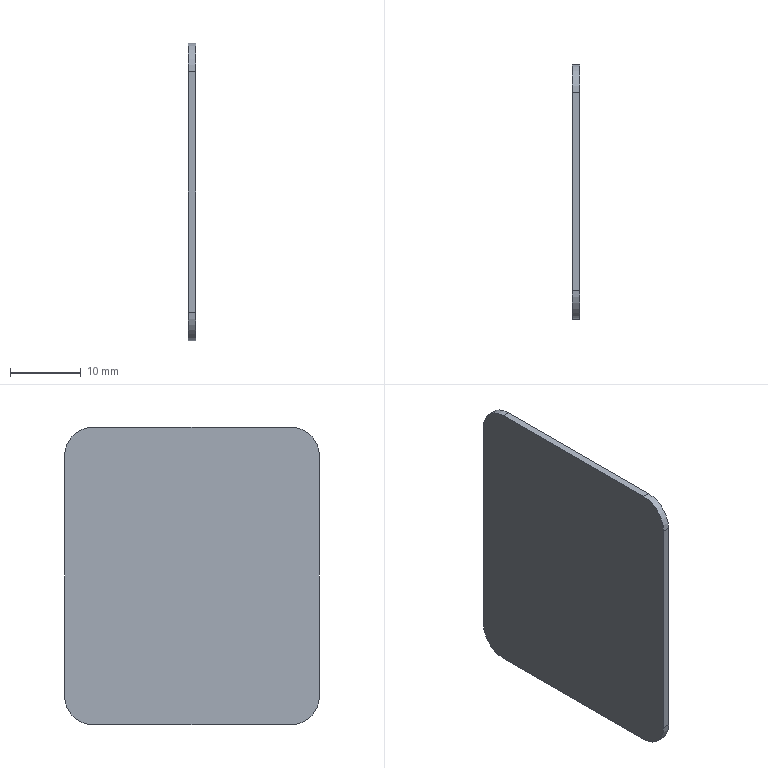Part | STEP file | 1-31.6 | 1 solid | 10 faces | box 1 x 36 x 42 mm | volume 1498 mm3 | plane 6 | cylinder 4 | commonest cylinder face diameters 8 x4
STEP:
#1=CARTESIAN_POINT('',(0.,0.,0.));
#2=DIRECTION('',(0.,0.,1.));
#3=DIRECTION('',(1.,0.,0.));
#4=AXIS2_PLACEMENT_3D('',#1,#2,#3);
#5=CARTESIAN_POINT('',(0.,18.,-17.));
#6=VERTEX_POINT('',#5);
#7=CARTESIAN_POINT('',(0.,18.,17.));
#8=VERTEX_POINT('',#7);
#9=CARTESIAN_POINT('',(0.,18.,-17.));
#10=DIRECTION('',(0.,0.,1.));
#11=VECTOR('',#10,1.);
#12=LINE('',#9,#11);
#13=CARTESIAN_POINT('',(0.,3.,0.));
#14=DIRECTION('',(1.,0.,0.));
#15=DIRECTION('',(0.,1.,0.));
#16=AXIS2_PLACEMENT_3D('',#13,#14,#15);
#17=PLANE('',#16);
#18=CARTESIAN_POINT('',(15.,-17.));
#19=DIRECTION('',(0.,1.));
#20=VECTOR('',#19,1.);
#21=LINE('',#18,#20);
#22=(GEOMETRIC_REPRESENTATION_CONTEXT(2)PARAMETRIC_REPRESENTATION_CONTEXT()REPRESENTATION_CONTEXT('',''));
#23=DEFINITIONAL_REPRESENTATION('',(#21),#22);
#24=PCURVE('',#17,#23);
#25=CARTESIAN_POINT('',(-0.5,18.,0.));
#26=DIRECTION('',(0.,-1.,0.));
#27=DIRECTION('',(0.,0.,1.));
#28=AXIS2_PLACEMENT_3D('',#25,#26,#27);
#29=PLANE('',#28);
#30=CARTESIAN_POINT('',(-17.,-0.5));
#31=DIRECTION('',(1.,0.));
#32=VECTOR('',#31,1.);
#33=LINE('',#30,#32);
#34=(GEOMETRIC_REPRESENTATION_CONTEXT(2)PARAMETRIC_REPRESENTATION_CONTEXT()REPRESENTATION_CONTEXT('',''));
#35=DEFINITIONAL_REPRESENTATION('',(#33),#34);
#36=PCURVE('',#29,#35);
#37=SURFACE_CURVE('',#12,(#24,#36),.PCURVE_S1.);
#38=EDGE_CURVE('',#6,#8,#37,.T.);
#39=ORIENTED_EDGE('',*,*,#38,.T.);
#40=CARTESIAN_POINT('',(0.,14.,21.));
#41=VERTEX_POINT('',#40);
#42=CARTESIAN_POINT('',(0.,14.,17.));
#43=DIRECTION('',(1.,0.,0.));
#44=DIRECTION('',(0.,1.,0.));
#45=AXIS2_PLACEMENT_3D('',#42,#43,#44);
#46=CIRCLE('',#45,4.);
#47=CARTESIAN_POINT('',(11.,17.));
#48=DIRECTION('',(1.,0.));
#49=AXIS2_PLACEMENT_2D('',#47,#48);
#50=CIRCLE('',#49,4.);
#51=(GEOMETRIC_REPRESENTATION_CONTEXT(2)PARAMETRIC_REPRESENTATION_CONTEXT()REPRESENTATION_CONTEXT('',''));
#52=DEFINITIONAL_REPRESENTATION('',(#50),#51);
#53=PCURVE('',#17,#52);
#54=CARTESIAN_POINT('',(0.,14.,17.));
#55=DIRECTION('',(-1.,0.,0.));
#56=DIRECTION('',(0.,1.,0.));
#57=AXIS2_PLACEMENT_3D('',#54,#55,#56);
#58=CYLINDRICAL_SURFACE('',#57,4.);
#59=CARTESIAN_POINT('',(6.283,0.));
#60=DIRECTION('',(-1.,0.));
#61=VECTOR('',#60,1.);
#62=LINE('',#59,#61);
#63=(GEOMETRIC_REPRESENTATION_CONTEXT(2)PARAMETRIC_REPRESENTATION_CONTEXT()REPRESENTATION_CONTEXT('',''));
#64=DEFINITIONAL_REPRESENTATION('',(#62),#63);
#65=PCURVE('',#58,#64);
#66=SURFACE_CURVE('',#46,(#53,#65),.PCURVE_S1.);
#67=EDGE_CURVE('',#8,#41,#66,.T.);
#68=ORIENTED_EDGE('',*,*,#67,.T.);
#69=CARTESIAN_POINT('',(0.,-14.,21.));
#70=VERTEX_POINT('',#69);
#71=CARTESIAN_POINT('',(0.,14.,21.));
#72=DIRECTION('',(0.,-1.,0.));
#73=VECTOR('',#72,1.);
#74=LINE('',#71,#73);
#75=CARTESIAN_POINT('',(11.,21.));
#76=DIRECTION('',(-1.,0.));
#77=VECTOR('',#76,1.);
#78=LINE('',#75,#77);
#79=(GEOMETRIC_REPRESENTATION_CONTEXT(2)PARAMETRIC_REPRESENTATION_CONTEXT()REPRESENTATION_CONTEXT('',''));
#80=DEFINITIONAL_REPRESENTATION('',(#78),#79);
#81=PCURVE('',#17,#80);
#82=CARTESIAN_POINT('',(-0.5,0.,21.));
#83=DIRECTION('',(0.,0.,-1.));
#84=DIRECTION('',(0.,-1.,0.));
#85=AXIS2_PLACEMENT_3D('',#82,#83,#84);
#86=PLANE('',#85);
#87=CARTESIAN_POINT('',(-14.,-0.5));
#88=DIRECTION('',(1.,0.));
#89=VECTOR('',#88,1.);
#90=LINE('',#87,#89);
#91=(GEOMETRIC_REPRESENTATION_CONTEXT(2)PARAMETRIC_REPRESENTATION_CONTEXT()REPRESENTATION_CONTEXT('',''));
#92=DEFINITIONAL_REPRESENTATION('',(#90),#91);
#93=PCURVE('',#86,#92);
#94=SURFACE_CURVE('',#74,(#81,#93),.PCURVE_S1.);
#95=EDGE_CURVE('',#41,#70,#94,.T.);
#96=ORIENTED_EDGE('',*,*,#95,.T.);
#97=CARTESIAN_POINT('',(0.,-18.,17.));
#98=VERTEX_POINT('',#97);
#99=CARTESIAN_POINT('',(0.,-14.,17.));
#100=DIRECTION('',(1.,0.,0.));
#101=DIRECTION('',(0.,0.,1.));
#102=AXIS2_PLACEMENT_3D('',#99,#100,#101);
#103=CIRCLE('',#102,4.);
#104=CARTESIAN_POINT('',(-17.,17.));
#105=DIRECTION('',(0.,1.));
#106=AXIS2_PLACEMENT_2D('',#104,#105);
#107=CIRCLE('',#106,4.);
#108=(GEOMETRIC_REPRESENTATION_CONTEXT(2)PARAMETRIC_REPRESENTATION_CONTEXT()REPRESENTATION_CONTEXT('',''));
#109=DEFINITIONAL_REPRESENTATION('',(#107),#108);
#110=PCURVE('',#17,#109);
#111=CARTESIAN_POINT('',(0.,-14.,17.));
#112=DIRECTION('',(-1.,0.,0.));
#113=DIRECTION('',(0.,0.,1.));
#114=AXIS2_PLACEMENT_3D('',#111,#112,#113);
#115=CYLINDRICAL_SURFACE('',#114,4.);
#116=CARTESIAN_POINT('',(6.283,0.));
#117=DIRECTION('',(-1.,0.));
#118=VECTOR('',#117,1.);
#119=LINE('',#116,#118);
#120=(GEOMETRIC_REPRESENTATION_CONTEXT(2)PARAMETRIC_REPRESENTATION_CONTEXT()REPRESENTATION_CONTEXT('',''));
#121=DEFINITIONAL_REPRESENTATION('',(#119),#120);
#122=PCURVE('',#115,#121);
#123=SURFACE_CURVE('',#103,(#110,#122),.PCURVE_S1.);
#124=EDGE_CURVE('',#70,#98,#123,.T.);
#125=ORIENTED_EDGE('',*,*,#124,.T.);
#126=CARTESIAN_POINT('',(0.,-18.,-17.));
#127=VERTEX_POINT('',#126);
#128=CARTESIAN_POINT('',(0.,-18.,17.));
#129=DIRECTION('',(0.,0.,-1.));
#130=VECTOR('',#129,1.);
#131=LINE('',#128,#130);
#132=CARTESIAN_POINT('',(-21.,17.));
#133=DIRECTION('',(0.,-1.));
#134=VECTOR('',#133,1.);
#135=LINE('',#132,#134);
#136=(GEOMETRIC_REPRESENTATION_CONTEXT(2)PARAMETRIC_REPRESENTATION_CONTEXT()REPRESENTATION_CONTEXT('',''));
#137=DEFINITIONAL_REPRESENTATION('',(#135),#136);
#138=PCURVE('',#17,#137);
#139=CARTESIAN_POINT('',(-0.5,-18.,0.));
#140=DIRECTION('',(0.,1.,0.));
#141=DIRECTION('',(0.,0.,-1.));
#142=AXIS2_PLACEMENT_3D('',#139,#140,#141);
#143=PLANE('',#142);
#144=CARTESIAN_POINT('',(-17.,-0.5));
#145=DIRECTION('',(1.,0.));
#146=VECTOR('',#145,1.);
#147=LINE('',#144,#146);
#148=(GEOMETRIC_REPRESENTATION_CONTEXT(2)PARAMETRIC_REPRESENTATION_CONTEXT()REPRESENTATION_CONTEXT('',''));
#149=DEFINITIONAL_REPRESENTATION('',(#147),#148);
#150=PCURVE('',#143,#149);
#151=SURFACE_CURVE('',#131,(#138,#150),.PCURVE_S1.);
#152=EDGE_CURVE('',#98,#127,#151,.T.);
#153=ORIENTED_EDGE('',*,*,#152,.T.);
#154=CARTESIAN_POINT('',(0.,-14.,-21.));
#155=VERTEX_POINT('',#154);
#156=CARTESIAN_POINT('',(0.,-14.,-17.));
#157=DIRECTION('',(1.,0.,0.));
#158=DIRECTION('',(0.,-1.,0.));
#159=AXIS2_PLACEMENT_3D('',#156,#157,#158);
#160=CIRCLE('',#159,4.);
#161=CARTESIAN_POINT('',(-17.,-17.));
#162=DIRECTION('',(-1.,0.));
#163=AXIS2_PLACEMENT_2D('',#161,#162);
#164=CIRCLE('',#163,4.);
#165=(GEOMETRIC_REPRESENTATION_CONTEXT(2)PARAMETRIC_REPRESENTATION_CONTEXT()REPRESENTATION_CONTEXT('',''));
#166=DEFINITIONAL_REPRESENTATION('',(#164),#165);
#167=PCURVE('',#17,#166);
#168=CARTESIAN_POINT('',(0.,-14.,-17.));
#169=DIRECTION('',(-1.,0.,0.));
#170=DIRECTION('',(0.,-1.,0.));
#171=AXIS2_PLACEMENT_3D('',#168,#169,#170);
#172=CYLINDRICAL_SURFACE('',#171,4.);
#173=CARTESIAN_POINT('',(6.283,0.));
#174=DIRECTION('',(-1.,0.));
#175=VECTOR('',#174,1.);
#176=LINE('',#173,#175);
#177=(GEOMETRIC_REPRESENTATION_CONTEXT(2)PARAMETRIC_REPRESENTATION_CONTEXT()REPRESENTATION_CONTEXT('',''));
#178=DEFINITIONAL_REPRESENTATION('',(#176),#177);
#179=PCURVE('',#172,#178);
#180=SURFACE_CURVE('',#160,(#167,#179),.PCURVE_S1.);
#181=EDGE_CURVE('',#127,#155,#180,.T.);
#182=ORIENTED_EDGE('',*,*,#181,.T.);
#183=CARTESIAN_POINT('',(0.,14.,-21.));
#184=VERTEX_POINT('',#183);
#185=CARTESIAN_POINT('',(0.,-14.,-21.));
#186=DIRECTION('',(0.,1.,0.));
#187=VECTOR('',#186,1.);
#188=LINE('',#185,#187);
#189=CARTESIAN_POINT('',(-17.,-21.));
#190=DIRECTION('',(1.,0.));
#191=VECTOR('',#190,1.);
#192=LINE('',#189,#191);
#193=(GEOMETRIC_REPRESENTATION_CONTEXT(2)PARAMETRIC_REPRESENTATION_CONTEXT()REPRESENTATION_CONTEXT('',''));
#194=DEFINITIONAL_REPRESENTATION('',(#192),#193);
#195=PCURVE('',#17,#194);
#196=CARTESIAN_POINT('',(-0.5,0.,-21.));
#197=DIRECTION('',(0.,0.,1.));
#198=DIRECTION('',(0.,1.,0.));
#199=AXIS2_PLACEMENT_3D('',#196,#197,#198);
#200=PLANE('',#199);
#201=CARTESIAN_POINT('',(-14.,-0.5));
#202=DIRECTION('',(1.,0.));
#203=VECTOR('',#202,1.);
#204=LINE('',#201,#203);
#205=(GEOMETRIC_REPRESENTATION_CONTEXT(2)PARAMETRIC_REPRESENTATION_CONTEXT()REPRESENTATION_CONTEXT('',''));
#206=DEFINITIONAL_REPRESENTATION('',(#204),#205);
#207=PCURVE('',#200,#206);
#208=SURFACE_CURVE('',#188,(#195,#207),.PCURVE_S1.);
#209=EDGE_CURVE('',#155,#184,#208,.T.);
#210=ORIENTED_EDGE('',*,*,#209,.T.);
#211=CARTESIAN_POINT('',(0.,14.,-17.));
#212=DIRECTION('',(1.,0.,0.));
#213=DIRECTION('',(0.,0.,-1.));
#214=AXIS2_PLACEMENT_3D('',#211,#212,#213);
#215=CIRCLE('',#214,4.);
#216=CARTESIAN_POINT('',(11.,-17.));
#217=DIRECTION('',(0.,-1.));
#218=AXIS2_PLACEMENT_2D('',#216,#217);
#219=CIRCLE('',#218,4.);
#220=(GEOMETRIC_REPRESENTATION_CONTEXT(2)PARAMETRIC_REPRESENTATION_CONTEXT()REPRESENTATION_CONTEXT('',''));
#221=DEFINITIONAL_REPRESENTATION('',(#219),#220);
#222=PCURVE('',#17,#221);
#223=CARTESIAN_POINT('',(0.,14.,-17.));
#224=DIRECTION('',(-1.,0.,0.));
#225=DIRECTION('',(0.,0.,-1.));
#226=AXIS2_PLACEMENT_3D('',#223,#224,#225);
#227=CYLINDRICAL_SURFACE('',#226,4.);
#228=CARTESIAN_POINT('',(6.283,0.));
#229=DIRECTION('',(-1.,0.));
#230=VECTOR('',#229,1.);
#231=LINE('',#228,#230);
#232=(GEOMETRIC_REPRESENTATION_CONTEXT(2)PARAMETRIC_REPRESENTATION_CONTEXT()REPRESENTATION_CONTEXT('',''));
#233=DEFINITIONAL_REPRESENTATION('',(#231),#232);
#234=PCURVE('',#227,#233);
#235=SURFACE_CURVE('',#215,(#222,#234),.PCURVE_S1.);
#236=EDGE_CURVE('',#184,#6,#235,.T.);
#237=ORIENTED_EDGE('',*,*,#236,.T.);
#238=EDGE_LOOP('',(#39,#68,#96,#125,#153,#182,#210,#237));
#239=FACE_BOUND('',#238,.T.);
#240=ADVANCED_FACE('',(#239),#17,.T.);
#241=CARTESIAN_POINT('',(-1.,18.,-17.));
#242=VERTEX_POINT('',#241);
#243=CARTESIAN_POINT('',(-1.,18.,17.));
#244=VERTEX_POINT('',#243);
#245=CARTESIAN_POINT('',(-1.,18.,-17.));
#246=DIRECTION('',(0.,0.,1.));
#247=VECTOR('',#246,1.);
#248=LINE('',#245,#247);
#249=CARTESIAN_POINT('',(-1.,3.,0.));
#250=DIRECTION('',(1.,0.,0.));
#251=DIRECTION('',(0.,1.,0.));
#252=AXIS2_PLACEMENT_3D('',#249,#250,#251);
#253=PLANE('',#252);
#254=CARTESIAN_POINT('',(15.,-17.));
#255=DIRECTION('',(0.,1.));
#256=VECTOR('',#255,1.);
#257=LINE('',#254,#256);
#258=(GEOMETRIC_REPRESENTATION_CONTEXT(2)PARAMETRIC_REPRESENTATION_CONTEXT()REPRESENTATION_CONTEXT('',''));
#259=DEFINITIONAL_REPRESENTATION('',(#257),#258);
#260=PCURVE('',#253,#259);
#261=CARTESIAN_POINT('',(-17.,0.5));
#262=DIRECTION('',(1.,0.));
#263=VECTOR('',#262,1.);
#264=LINE('',#261,#263);
#265=(GEOMETRIC_REPRESENTATION_CONTEXT(2)PARAMETRIC_REPRESENTATION_CONTEXT()REPRESENTATION_CONTEXT('',''));
#266=DEFINITIONAL_REPRESENTATION('',(#264),#265);
#267=PCURVE('',#29,#266);
#268=SURFACE_CURVE('',#248,(#260,#267),.PCURVE_S1.);
#269=EDGE_CURVE('',#242,#244,#268,.T.);
#270=ORIENTED_EDGE('',*,*,#269,.T.);
#271=CARTESIAN_POINT('',(-1.,14.,21.));
#272=VERTEX_POINT('',#271);
#273=CARTESIAN_POINT('',(-1.,14.,17.));
#274=DIRECTION('',(1.,0.,0.));
#275=DIRECTION('',(0.,1.,0.));
#276=AXIS2_PLACEMENT_3D('',#273,#274,#275);
#277=CIRCLE('',#276,4.);
#278=CARTESIAN_POINT('',(11.,17.));
#279=DIRECTION('',(1.,0.));
#280=AXIS2_PLACEMENT_2D('',#278,#279);
#281=CIRCLE('',#280,4.);
#282=(GEOMETRIC_REPRESENTATION_CONTEXT(2)PARAMETRIC_REPRESENTATION_CONTEXT()REPRESENTATION_CONTEXT('',''));
#283=DEFINITIONAL_REPRESENTATION('',(#281),#282);
#284=PCURVE('',#253,#283);
#285=CARTESIAN_POINT('',(6.283,1.));
#286=DIRECTION('',(-1.,0.));
#287=VECTOR('',#286,1.);
#288=LINE('',#285,#287);
#289=(GEOMETRIC_REPRESENTATION_CONTEXT(2)PARAMETRIC_REPRESENTATION_CONTEXT()REPRESENTATION_CONTEXT('',''));
#290=DEFINITIONAL_REPRESENTATION('',(#288),#289);
#291=PCURVE('',#58,#290);
#292=SURFACE_CURVE('',#277,(#284,#291),.PCURVE_S1.);
#293=EDGE_CURVE('',#244,#272,#292,.T.);
#294=ORIENTED_EDGE('',*,*,#293,.T.);
#295=CARTESIAN_POINT('',(-1.,-14.,21.));
#296=VERTEX_POINT('',#295);
#297=CARTESIAN_POINT('',(-1.,14.,21.));
#298=DIRECTION('',(0.,-1.,0.));
#299=VECTOR('',#298,1.);
#300=LINE('',#297,#299);
#301=CARTESIAN_POINT('',(11.,21.));
#302=DIRECTION('',(-1.,0.));
#303=VECTOR('',#302,1.);
#304=LINE('',#301,#303);
#305=(GEOMETRIC_REPRESENTATION_CONTEXT(2)PARAMETRIC_REPRESENTATION_CONTEXT()REPRESENTATION_CONTEXT('',''));
#306=DEFINITIONAL_REPRESENTATION('',(#304),#305);
#307=PCURVE('',#253,#306);
#308=CARTESIAN_POINT('',(-14.,0.5));
#309=DIRECTION('',(1.,0.));
#310=VECTOR('',#309,1.);
#311=LINE('',#308,#310);
#312=(GEOMETRIC_REPRESENTATION_CONTEXT(2)PARAMETRIC_REPRESENTATION_CONTEXT()REPRESENTATION_CONTEXT('',''));
#313=DEFINITIONAL_REPRESENTATION('',(#311),#312);
#314=PCURVE('',#86,#313);
#315=SURFACE_CURVE('',#300,(#307,#314),.PCURVE_S1.);
#316=EDGE_CURVE('',#272,#296,#315,.T.);
#317=ORIENTED_EDGE('',*,*,#316,.T.);
#318=CARTESIAN_POINT('',(-1.,-18.,17.));
#319=VERTEX_POINT('',#318);
#320=CARTESIAN_POINT('',(-1.,-14.,17.));
#321=DIRECTION('',(1.,0.,0.));
#322=DIRECTION('',(0.,0.,1.));
#323=AXIS2_PLACEMENT_3D('',#320,#321,#322);
#324=CIRCLE('',#323,4.);
#325=CARTESIAN_POINT('',(-17.,17.));
#326=DIRECTION('',(0.,1.));
#327=AXIS2_PLACEMENT_2D('',#325,#326);
#328=CIRCLE('',#327,4.);
#329=(GEOMETRIC_REPRESENTATION_CONTEXT(2)PARAMETRIC_REPRESENTATION_CONTEXT()REPRESENTATION_CONTEXT('',''));
#330=DEFINITIONAL_REPRESENTATION('',(#328),#329);
#331=PCURVE('',#253,#330);
#332=CARTESIAN_POINT('',(6.283,1.));
#333=DIRECTION('',(-1.,0.));
#334=VECTOR('',#333,1.);
#335=LINE('',#332,#334);
#336=(GEOMETRIC_REPRESENTATION_CONTEXT(2)PARAMETRIC_REPRESENTATION_CONTEXT()REPRESENTATION_CONTEXT('',''));
#337=DEFINITIONAL_REPRESENTATION('',(#335),#336);
#338=PCURVE('',#115,#337);
#339=SURFACE_CURVE('',#324,(#331,#338),.PCURVE_S1.);
#340=EDGE_CURVE('',#296,#319,#339,.T.);
#341=ORIENTED_EDGE('',*,*,#340,.T.);
#342=CARTESIAN_POINT('',(-1.,-18.,-17.));
#343=VERTEX_POINT('',#342);
#344=CARTESIAN_POINT('',(-1.,-18.,17.));
#345=DIRECTION('',(0.,0.,-1.));
#346=VECTOR('',#345,1.);
#347=LINE('',#344,#346);
#348=CARTESIAN_POINT('',(-21.,17.));
#349=DIRECTION('',(0.,-1.));
#350=VECTOR('',#349,1.);
#351=LINE('',#348,#350);
#352=(GEOMETRIC_REPRESENTATION_CONTEXT(2)PARAMETRIC_REPRESENTATION_CONTEXT()REPRESENTATION_CONTEXT('',''));
#353=DEFINITIONAL_REPRESENTATION('',(#351),#352);
#354=PCURVE('',#253,#353);
#355=CARTESIAN_POINT('',(-17.,0.5));
#356=DIRECTION('',(1.,0.));
#357=VECTOR('',#356,1.);
#358=LINE('',#355,#357);
#359=(GEOMETRIC_REPRESENTATION_CONTEXT(2)PARAMETRIC_REPRESENTATION_CONTEXT()REPRESENTATION_CONTEXT('',''));
#360=DEFINITIONAL_REPRESENTATION('',(#358),#359);
#361=PCURVE('',#143,#360);
#362=SURFACE_CURVE('',#347,(#354,#361),.PCURVE_S1.);
#363=EDGE_CURVE('',#319,#343,#362,.T.);
#364=ORIENTED_EDGE('',*,*,#363,.T.);
#365=CARTESIAN_POINT('',(-1.,-14.,-21.));
#366=VERTEX_POINT('',#365);
#367=CARTESIAN_POINT('',(-1.,-14.,-17.));
#368=DIRECTION('',(1.,0.,0.));
#369=DIRECTION('',(0.,-1.,0.));
#370=AXIS2_PLACEMENT_3D('',#367,#368,#369);
#371=CIRCLE('',#370,4.);
#372=CARTESIAN_POINT('',(-17.,-17.));
#373=DIRECTION('',(-1.,0.));
#374=AXIS2_PLACEMENT_2D('',#372,#373);
#375=CIRCLE('',#374,4.);
#376=(GEOMETRIC_REPRESENTATION_CONTEXT(2)PARAMETRIC_REPRESENTATION_CONTEXT()REPRESENTATION_CONTEXT('',''));
#377=DEFINITIONAL_REPRESENTATION('',(#375),#376);
#378=PCURVE('',#253,#377);
#379=CARTESIAN_POINT('',(6.283,1.));
#380=DIRECTION('',(-1.,0.));
#381=VECTOR('',#380,1.);
#382=LINE('',#379,#381);
#383=(GEOMETRIC_REPRESENTATION_CONTEXT(2)PARAMETRIC_REPRESENTATION_CONTEXT()REPRESENTATION_CONTEXT('',''));
#384=DEFINITIONAL_REPRESENTATION('',(#382),#383);
#385=PCURVE('',#172,#384);
#386=SURFACE_CURVE('',#371,(#378,#385),.PCURVE_S1.);
#387=EDGE_CURVE('',#343,#366,#386,.T.);
#388=ORIENTED_EDGE('',*,*,#387,.T.);
#389=CARTESIAN_POINT('',(-1.,14.,-21.));
#390=VERTEX_POINT('',#389);
#391=CARTESIAN_POINT('',(-1.,-14.,-21.));
#392=DIRECTION('',(0.,1.,0.));
#393=VECTOR('',#392,1.);
#394=LINE('',#391,#393);
#395=CARTESIAN_POINT('',(-17.,-21.));
#396=DIRECTION('',(1.,0.));
#397=VECTOR('',#396,1.);
#398=LINE('',#395,#397);
#399=(GEOMETRIC_REPRESENTATION_CONTEXT(2)PARAMETRIC_REPRESENTATION_CONTEXT()REPRESENTATION_CONTEXT('',''));
#400=DEFINITIONAL_REPRESENTATION('',(#398),#399);
#401=PCURVE('',#253,#400);
#402=CARTESIAN_POINT('',(-14.,0.5));
#403=DIRECTION('',(1.,0.));
#404=VECTOR('',#403,1.);
#405=LINE('',#402,#404);
#406=(GEOMETRIC_REPRESENTATION_CONTEXT(2)PARAMETRIC_REPRESENTATION_CONTEXT()REPRESENTATION_CONTEXT('',''));
#407=DEFINITIONAL_REPRESENTATION('',(#405),#406);
#408=PCURVE('',#200,#407);
#409=SURFACE_CURVE('',#394,(#401,#408),.PCURVE_S1.);
#410=EDGE_CURVE('',#366,#390,#409,.T.);
#411=ORIENTED_EDGE('',*,*,#410,.T.);
#412=CARTESIAN_POINT('',(-1.,14.,-17.));
#413=DIRECTION('',(1.,0.,0.));
#414=DIRECTION('',(0.,0.,-1.));
#415=AXIS2_PLACEMENT_3D('',#412,#413,#414);
#416=CIRCLE('',#415,4.);
#417=CARTESIAN_POINT('',(11.,-17.));
#418=DIRECTION('',(0.,-1.));
#419=AXIS2_PLACEMENT_2D('',#417,#418);
#420=CIRCLE('',#419,4.);
#421=(GEOMETRIC_REPRESENTATION_CONTEXT(2)PARAMETRIC_REPRESENTATION_CONTEXT()REPRESENTATION_CONTEXT('',''));
#422=DEFINITIONAL_REPRESENTATION('',(#420),#421);
#423=PCURVE('',#253,#422);
#424=CARTESIAN_POINT('',(6.283,1.));
#425=DIRECTION('',(-1.,0.));
#426=VECTOR('',#425,1.);
#427=LINE('',#424,#426);
#428=(GEOMETRIC_REPRESENTATION_CONTEXT(2)PARAMETRIC_REPRESENTATION_CONTEXT()REPRESENTATION_CONTEXT('',''));
#429=DEFINITIONAL_REPRESENTATION('',(#427),#428);
#430=PCURVE('',#227,#429);
#431=SURFACE_CURVE('',#416,(#423,#430),.PCURVE_S1.);
#432=EDGE_CURVE('',#390,#242,#431,.T.);
#433=ORIENTED_EDGE('',*,*,#432,.T.);
#434=EDGE_LOOP('',(#270,#294,#317,#341,#364,#388,#411,#433));
#435=FACE_BOUND('',#434,.F.);
#436=ADVANCED_FACE('',(#435),#253,.F.);
#437=ORIENTED_EDGE('',*,*,#410,.F.);
#438=CARTESIAN_POINT('',(0.,-14.,-21.));
#439=DIRECTION('',(-1.,0.,0.));
#440=VECTOR('',#439,1.);
#441=LINE('',#438,#440);
#442=CARTESIAN_POINT('',(-14.,-0.5));
#443=DIRECTION('',(0.,1.));
#444=VECTOR('',#443,1.);
#445=LINE('',#442,#444);
#446=(GEOMETRIC_REPRESENTATION_CONTEXT(2)PARAMETRIC_REPRESENTATION_CONTEXT()REPRESENTATION_CONTEXT('',''));
#447=DEFINITIONAL_REPRESENTATION('',(#445),#446);
#448=PCURVE('',#200,#447);
#449=CARTESIAN_POINT('',(4.712,0.));
#450=DIRECTION('',(0.,1.));
#451=VECTOR('',#450,1.);
#452=LINE('',#449,#451);
#453=(GEOMETRIC_REPRESENTATION_CONTEXT(2)PARAMETRIC_REPRESENTATION_CONTEXT()REPRESENTATION_CONTEXT('',''));
#454=DEFINITIONAL_REPRESENTATION('',(#452),#453);
#455=PCURVE('',#172,#454);
#456=SURFACE_CURVE('',#441,(#448,#455),.PCURVE_S1.);
#457=EDGE_CURVE('',#155,#366,#456,.T.);
#458=ORIENTED_EDGE('',*,*,#457,.F.);
#459=ORIENTED_EDGE('',*,*,#209,.T.);
#460=CARTESIAN_POINT('',(0.,14.,-21.));
#461=DIRECTION('',(-1.,0.,0.));
#462=VECTOR('',#461,1.);
#463=LINE('',#460,#462);
#464=CARTESIAN_POINT('',(14.,-0.5));
#465=DIRECTION('',(0.,1.));
#466=VECTOR('',#465,1.);
#467=LINE('',#464,#466);
#468=(GEOMETRIC_REPRESENTATION_CONTEXT(2)PARAMETRIC_REPRESENTATION_CONTEXT()REPRESENTATION_CONTEXT('',''));
#469=DEFINITIONAL_REPRESENTATION('',(#467),#468);
#470=PCURVE('',#200,#469);
#471=CARTESIAN_POINT('',(6.283,0.));
#472=DIRECTION('',(0.,1.));
#473=VECTOR('',#472,1.);
#474=LINE('',#471,#473);
#475=(GEOMETRIC_REPRESENTATION_CONTEXT(2)PARAMETRIC_REPRESENTATION_CONTEXT()REPRESENTATION_CONTEXT('',''));
#476=DEFINITIONAL_REPRESENTATION('',(#474),#475);
#477=PCURVE('',#227,#476);
#478=SURFACE_CURVE('',#463,(#470,#477),.PCURVE_S1.);
#479=EDGE_CURVE('',#184,#390,#478,.T.);
#480=ORIENTED_EDGE('',*,*,#479,.T.);
#481=EDGE_LOOP('',(#437,#458,#459,#480));
#482=FACE_BOUND('',#481,.F.);
#483=ADVANCED_FACE('',(#482),#200,.F.);
#484=ORIENTED_EDGE('',*,*,#38,.T.);
#485=CARTESIAN_POINT('',(0.,18.,17.));
#486=DIRECTION('',(-1.,0.,0.));
#487=VECTOR('',#486,1.);
#488=LINE('',#485,#487);
#489=CARTESIAN_POINT('',(17.,-0.5));
#490=DIRECTION('',(0.,1.));
#491=VECTOR('',#490,1.);
#492=LINE('',#489,#491);
#493=(GEOMETRIC_REPRESENTATION_CONTEXT(2)PARAMETRIC_REPRESENTATION_CONTEXT()REPRESENTATION_CONTEXT('',''));
#494=DEFINITIONAL_REPRESENTATION('',(#492),#493);
#495=PCURVE('',#29,#494);
#496=CARTESIAN_POINT('',(6.283,0.));
#497=DIRECTION('',(0.,1.));
#498=VECTOR('',#497,1.);
#499=LINE('',#496,#498);
#500=(GEOMETRIC_REPRESENTATION_CONTEXT(2)PARAMETRIC_REPRESENTATION_CONTEXT()REPRESENTATION_CONTEXT('',''));
#501=DEFINITIONAL_REPRESENTATION('',(#499),#500);
#502=PCURVE('',#58,#501);
#503=SURFACE_CURVE('',#488,(#495,#502),.PCURVE_S1.);
#504=EDGE_CURVE('',#8,#244,#503,.T.);
#505=ORIENTED_EDGE('',*,*,#504,.T.);
#506=ORIENTED_EDGE('',*,*,#269,.F.);
#507=CARTESIAN_POINT('',(0.,18.,-17.));
#508=DIRECTION('',(-1.,0.,0.));
#509=VECTOR('',#508,1.);
#510=LINE('',#507,#509);
#511=CARTESIAN_POINT('',(-17.,-0.5));
#512=DIRECTION('',(0.,1.));
#513=VECTOR('',#512,1.);
#514=LINE('',#511,#513);
#515=(GEOMETRIC_REPRESENTATION_CONTEXT(2)PARAMETRIC_REPRESENTATION_CONTEXT()REPRESENTATION_CONTEXT('',''));
#516=DEFINITIONAL_REPRESENTATION('',(#514),#515);
#517=PCURVE('',#29,#516);
#518=CARTESIAN_POINT('',(4.712,0.));
#519=DIRECTION('',(0.,1.));
#520=VECTOR('',#519,1.);
#521=LINE('',#518,#520);
#522=(GEOMETRIC_REPRESENTATION_CONTEXT(2)PARAMETRIC_REPRESENTATION_CONTEXT()REPRESENTATION_CONTEXT('',''));
#523=DEFINITIONAL_REPRESENTATION('',(#521),#522);
#524=PCURVE('',#227,#523);
#525=SURFACE_CURVE('',#510,(#517,#524),.PCURVE_S1.);
#526=EDGE_CURVE('',#6,#242,#525,.T.);
#527=ORIENTED_EDGE('',*,*,#526,.F.);
#528=EDGE_LOOP('',(#484,#505,#506,#527));
#529=FACE_BOUND('',#528,.F.);
#530=ADVANCED_FACE('',(#529),#29,.F.);
#531=ORIENTED_EDGE('',*,*,#95,.T.);
#532=CARTESIAN_POINT('',(0.,-14.,21.));
#533=DIRECTION('',(-1.,0.,0.));
#534=VECTOR('',#533,1.);
#535=LINE('',#532,#534);
#536=CARTESIAN_POINT('',(14.,-0.5));
#537=DIRECTION('',(0.,1.));
#538=VECTOR('',#537,1.);
#539=LINE('',#536,#538);
#540=(GEOMETRIC_REPRESENTATION_CONTEXT(2)PARAMETRIC_REPRESENTATION_CONTEXT()REPRESENTATION_CONTEXT('',''));
#541=DEFINITIONAL_REPRESENTATION('',(#539),#540);
#542=PCURVE('',#86,#541);
#543=CARTESIAN_POINT('',(6.283,0.));
#544=DIRECTION('',(0.,1.));
#545=VECTOR('',#544,1.);
#546=LINE('',#543,#545);
#547=(GEOMETRIC_REPRESENTATION_CONTEXT(2)PARAMETRIC_REPRESENTATION_CONTEXT()REPRESENTATION_CONTEXT('',''));
#548=DEFINITIONAL_REPRESENTATION('',(#546),#547);
#549=PCURVE('',#115,#548);
#550=SURFACE_CURVE('',#535,(#542,#549),.PCURVE_S1.);
#551=EDGE_CURVE('',#70,#296,#550,.T.);
#552=ORIENTED_EDGE('',*,*,#551,.T.);
#553=ORIENTED_EDGE('',*,*,#316,.F.);
#554=CARTESIAN_POINT('',(0.,14.,21.));
#555=DIRECTION('',(-1.,0.,0.));
#556=VECTOR('',#555,1.);
#557=LINE('',#554,#556);
#558=CARTESIAN_POINT('',(-14.,-0.5));
#559=DIRECTION('',(0.,1.));
#560=VECTOR('',#559,1.);
#561=LINE('',#558,#560);
#562=(GEOMETRIC_REPRESENTATION_CONTEXT(2)PARAMETRIC_REPRESENTATION_CONTEXT()REPRESENTATION_CONTEXT('',''));
#563=DEFINITIONAL_REPRESENTATION('',(#561),#562);
#564=PCURVE('',#86,#563);
#565=CARTESIAN_POINT('',(4.712,0.));
#566=DIRECTION('',(0.,1.));
#567=VECTOR('',#566,1.);
#568=LINE('',#565,#567);
#569=(GEOMETRIC_REPRESENTATION_CONTEXT(2)PARAMETRIC_REPRESENTATION_CONTEXT()REPRESENTATION_CONTEXT('',''));
#570=DEFINITIONAL_REPRESENTATION('',(#568),#569);
#571=PCURVE('',#58,#570);
#572=SURFACE_CURVE('',#557,(#564,#571),.PCURVE_S1.);
#573=EDGE_CURVE('',#41,#272,#572,.T.);
#574=ORIENTED_EDGE('',*,*,#573,.F.);
#575=EDGE_LOOP('',(#531,#552,#553,#574));
#576=FACE_BOUND('',#575,.F.);
#577=ADVANCED_FACE('',(#576),#86,.F.);
#578=ORIENTED_EDGE('',*,*,#152,.T.);
#579=CARTESIAN_POINT('',(0.,-18.,-17.));
#580=DIRECTION('',(-1.,0.,0.));
#581=VECTOR('',#580,1.);
#582=LINE('',#579,#581);
#583=CARTESIAN_POINT('',(17.,-0.5));
#584=DIRECTION('',(0.,1.));
#585=VECTOR('',#584,1.);
#586=LINE('',#583,#585);
#587=(GEOMETRIC_REPRESENTATION_CONTEXT(2)PARAMETRIC_REPRESENTATION_CONTEXT()REPRESENTATION_CONTEXT('',''));
#588=DEFINITIONAL_REPRESENTATION('',(#586),#587);
#589=PCURVE('',#143,#588);
#590=CARTESIAN_POINT('',(6.283,0.));
#591=DIRECTION('',(0.,1.));
#592=VECTOR('',#591,1.);
#593=LINE('',#590,#592);
#594=(GEOMETRIC_REPRESENTATION_CONTEXT(2)PARAMETRIC_REPRESENTATION_CONTEXT()REPRESENTATION_CONTEXT('',''));
#595=DEFINITIONAL_REPRESENTATION('',(#593),#594);
#596=PCURVE('',#172,#595);
#597=SURFACE_CURVE('',#582,(#589,#596),.PCURVE_S1.);
#598=EDGE_CURVE('',#127,#343,#597,.T.);
#599=ORIENTED_EDGE('',*,*,#598,.T.);
#600=ORIENTED_EDGE('',*,*,#363,.F.);
#601=CARTESIAN_POINT('',(0.,-18.,17.));
#602=DIRECTION('',(-1.,0.,0.));
#603=VECTOR('',#602,1.);
#604=LINE('',#601,#603);
#605=CARTESIAN_POINT('',(-17.,-0.5));
#606=DIRECTION('',(0.,1.));
#607=VECTOR('',#606,1.);
#608=LINE('',#605,#607);
#609=(GEOMETRIC_REPRESENTATION_CONTEXT(2)PARAMETRIC_REPRESENTATION_CONTEXT()REPRESENTATION_CONTEXT('',''));
#610=DEFINITIONAL_REPRESENTATION('',(#608),#609);
#611=PCURVE('',#143,#610);
#612=CARTESIAN_POINT('',(4.712,0.));
#613=DIRECTION('',(0.,1.));
#614=VECTOR('',#613,1.);
#615=LINE('',#612,#614);
#616=(GEOMETRIC_REPRESENTATION_CONTEXT(2)PARAMETRIC_REPRESENTATION_CONTEXT()REPRESENTATION_CONTEXT('',''));
#617=DEFINITIONAL_REPRESENTATION('',(#615),#616);
#618=PCURVE('',#115,#617);
#619=SURFACE_CURVE('',#604,(#611,#618),.PCURVE_S1.);
#620=EDGE_CURVE('',#98,#319,#619,.T.);
#621=ORIENTED_EDGE('',*,*,#620,.F.);
#622=EDGE_LOOP('',(#578,#599,#600,#621));
#623=FACE_BOUND('',#622,.F.);
#624=ADVANCED_FACE('',(#623),#143,.F.);
#625=ORIENTED_EDGE('',*,*,#504,.T.);
#626=ORIENTED_EDGE('',*,*,#293,.T.);
#627=ORIENTED_EDGE('',*,*,#573,.F.);
#628=ORIENTED_EDGE('',*,*,#67,.F.);
#629=EDGE_LOOP('',(#625,#626,#627,#628));
#630=FACE_BOUND('',#629,.T.);
#631=ADVANCED_FACE('',(#630),#58,.T.);
#632=ORIENTED_EDGE('',*,*,#551,.T.);
#633=ORIENTED_EDGE('',*,*,#340,.T.);
#634=ORIENTED_EDGE('',*,*,#620,.F.);
#635=ORIENTED_EDGE('',*,*,#124,.F.);
#636=EDGE_LOOP('',(#632,#633,#634,#635));
#637=FACE_BOUND('',#636,.T.);
#638=ADVANCED_FACE('',(#637),#115,.T.);
#639=ORIENTED_EDGE('',*,*,#598,.T.);
#640=ORIENTED_EDGE('',*,*,#387,.T.);
#641=ORIENTED_EDGE('',*,*,#457,.F.);
#642=ORIENTED_EDGE('',*,*,#181,.F.);
#643=EDGE_LOOP('',(#639,#640,#641,#642));
#644=FACE_BOUND('',#643,.T.);
#645=ADVANCED_FACE('',(#644),#172,.T.);
#646=ORIENTED_EDGE('',*,*,#479,.T.);
#647=ORIENTED_EDGE('',*,*,#432,.T.);
#648=ORIENTED_EDGE('',*,*,#526,.F.);
#649=ORIENTED_EDGE('',*,*,#236,.F.);
#650=EDGE_LOOP('',(#646,#647,#648,#649));
#651=FACE_BOUND('',#650,.T.);
#652=ADVANCED_FACE('',(#651),#227,.T.);
#653=CLOSED_SHELL('',(#240,#436,#483,#530,#577,#624,#631,#638,#645,#652));
#654=MANIFOLD_SOLID_BREP('',#653);
#655=(LENGTH_UNIT()NAMED_UNIT(*)SI_UNIT(.MILLI.,.METRE.));
#656=UNCERTAINTY_MEASURE_WITH_UNIT(LENGTH_MEASURE(0.0000001),#655,'','');
#657=(NAMED_UNIT(*)PLANE_ANGLE_UNIT()SI_UNIT($,.RADIAN.));
#658=(NAMED_UNIT(*)SI_UNIT($,.STERADIAN.)SOLID_ANGLE_UNIT());
#659=(GEOMETRIC_REPRESENTATION_CONTEXT(3)GLOBAL_UNCERTAINTY_ASSIGNED_CONTEXT((#656))GLOBAL_UNIT_ASSIGNED_CONTEXT((#655,#657,#658))REPRESENTATION_CONTEXT('',''));
#660=ADVANCED_BREP_SHAPE_REPRESENTATION('',(#4,#654),#659);